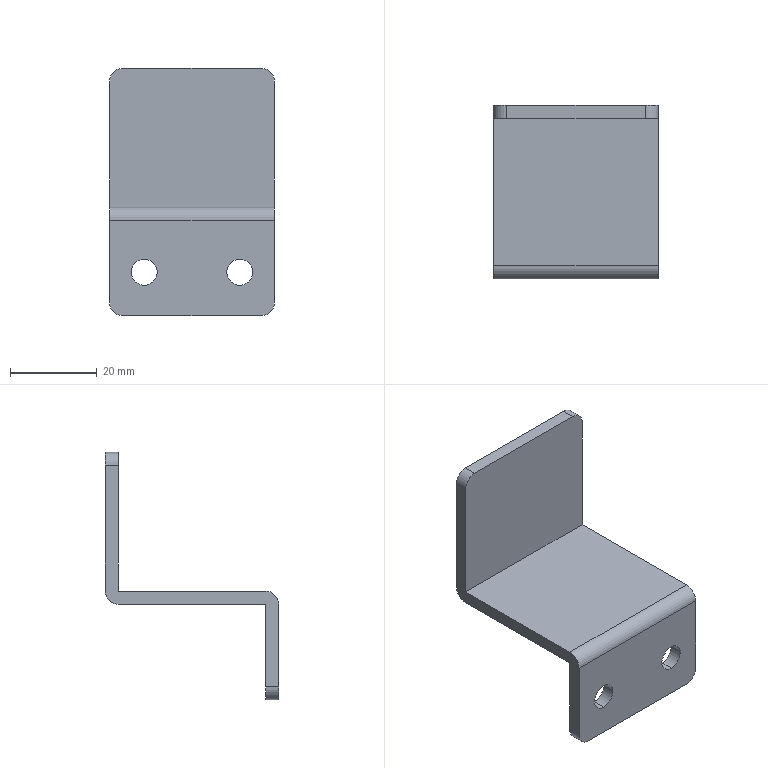Part | SolidWorks | features BaseBody 1 | 1 solid | 20 faces | box 38 x 40 x 57 mm | volume 10376 mm3 | cylinder 10 | plane 10 | commonest cylinder face diameters 6 x10
STEP:
#1=CARTESIAN_POINT('',(30.,-40.,-44.));
#2=VERTEX_POINT('',#1);
#3=CARTESIAN_POINT('',(30.,-40.,-50.));
#4=VERTEX_POINT('',#3);
#5=CARTESIAN_POINT('',(30.,-40.,-47.));
#6=DIRECTION('',(0.,-1.,0.));
#7=DIRECTION('',(0.,0.,1.));
#8=AXIS2_PLACEMENT_3D('',#5,#6,#7);
#9=CIRCLE('',#8,3.);
#10=EDGE_CURVE('',#2,#4,#9,.T.);
#11=ORIENTED_EDGE('',*,*,#10,.T.);
#12=CARTESIAN_POINT('',(30.,-37.,-50.));
#13=VERTEX_POINT('',#12);
#14=CARTESIAN_POINT('',(30.,-40.,-50.));
#15=DIRECTION('',(0.,1.,0.));
#16=VECTOR('',#15,1000.);
#17=LINE('',#14,#16);
#18=EDGE_CURVE('',#4,#13,#17,.T.);
#19=ORIENTED_EDGE('',*,*,#18,.T.);
#20=CARTESIAN_POINT('',(30.,-37.,-44.));
#21=VERTEX_POINT('',#20);
#22=CARTESIAN_POINT('',(30.,-37.,-47.));
#23=DIRECTION('',(0.,1.,0.));
#24=DIRECTION('',(0.,0.,1.));
#25=AXIS2_PLACEMENT_3D('',#22,#23,#24);
#26=CIRCLE('',#25,3.);
#27=EDGE_CURVE('',#13,#21,#26,.T.);
#28=ORIENTED_EDGE('',*,*,#27,.T.);
#29=CARTESIAN_POINT('',(30.,-40.,-44.));
#30=DIRECTION('',(0.,1.,0.));
#31=VECTOR('',#30,1000.);
#32=LINE('',#29,#31);
#33=EDGE_CURVE('',#2,#21,#32,.T.);
#34=ORIENTED_EDGE('',*,*,#33,.F.);
#35=EDGE_LOOP('',(#11,#19,#28,#34));
#36=FACE_OUTER_BOUND('',#35,.T.);
#37=CARTESIAN_POINT('',(30.,-40.,-47.));
#38=DIRECTION('',(0.,1.,0.));
#39=DIRECTION('',(0.,0.,1.));
#40=AXIS2_PLACEMENT_3D('',#37,#38,#39);
#41=CYLINDRICAL_SURFACE('',#40,3.);
#42=ADVANCED_FACE('',(#36),#41,.F.);
#43=CARTESIAN_POINT('',(8.,-40.,-44.));
#44=VERTEX_POINT('',#43);
#45=CARTESIAN_POINT('',(8.,-40.,-50.));
#46=VERTEX_POINT('',#45);
#47=CARTESIAN_POINT('',(8.,-40.,-47.));
#48=DIRECTION('',(0.,-1.,0.));
#49=DIRECTION('',(0.,0.,1.));
#50=AXIS2_PLACEMENT_3D('',#47,#48,#49);
#51=CIRCLE('',#50,3.);
#52=EDGE_CURVE('',#44,#46,#51,.T.);
#53=ORIENTED_EDGE('',*,*,#52,.T.);
#54=CARTESIAN_POINT('',(8.,-37.,-50.));
#55=VERTEX_POINT('',#54);
#56=CARTESIAN_POINT('',(8.,-40.,-50.));
#57=DIRECTION('',(0.,1.,0.));
#58=VECTOR('',#57,1000.);
#59=LINE('',#56,#58);
#60=EDGE_CURVE('',#46,#55,#59,.T.);
#61=ORIENTED_EDGE('',*,*,#60,.T.);
#62=CARTESIAN_POINT('',(8.,-37.,-44.));
#63=VERTEX_POINT('',#62);
#64=CARTESIAN_POINT('',(8.,-37.,-47.));
#65=DIRECTION('',(0.,1.,0.));
#66=DIRECTION('',(0.,0.,1.));
#67=AXIS2_PLACEMENT_3D('',#64,#65,#66);
#68=CIRCLE('',#67,3.);
#69=EDGE_CURVE('',#55,#63,#68,.T.);
#70=ORIENTED_EDGE('',*,*,#69,.T.);
#71=CARTESIAN_POINT('',(8.,-40.,-44.));
#72=DIRECTION('',(0.,1.,0.));
#73=VECTOR('',#72,1000.);
#74=LINE('',#71,#73);
#75=EDGE_CURVE('',#44,#63,#74,.T.);
#76=ORIENTED_EDGE('',*,*,#75,.F.);
#77=EDGE_LOOP('',(#53,#61,#70,#76));
#78=FACE_OUTER_BOUND('',#77,.T.);
#79=CARTESIAN_POINT('',(8.,-40.,-47.));
#80=DIRECTION('',(0.,1.,0.));
#81=DIRECTION('',(0.,0.,1.));
#82=AXIS2_PLACEMENT_3D('',#79,#80,#81);
#83=CYLINDRICAL_SURFACE('',#82,3.);
#84=ADVANCED_FACE('',(#78),#83,.F.);
#85=CARTESIAN_POINT('',(38.,-37.,-32.));
#86=VERTEX_POINT('',#85);
#87=CARTESIAN_POINT('',(0.,-37.,-32.));
#88=VERTEX_POINT('',#87);
#89=CARTESIAN_POINT('',(38.,-37.,-32.));
#90=DIRECTION('',(-1.,0.,0.));
#91=VECTOR('',#90,1000.);
#92=LINE('',#89,#91);
#93=EDGE_CURVE('',#86,#88,#92,.T.);
#94=ORIENTED_EDGE('',*,*,#93,.F.);
#95=CARTESIAN_POINT('',(38.,-3.,-32.));
#96=VERTEX_POINT('',#95);
#97=CARTESIAN_POINT('',(38.,-40.,-32.));
#98=DIRECTION('',(0.,-1.,0.));
#99=VECTOR('',#98,1000.);
#100=LINE('',#97,#99);
#101=EDGE_CURVE('',#96,#86,#100,.T.);
#102=ORIENTED_EDGE('',*,*,#101,.F.);
#103=CARTESIAN_POINT('',(0.,-3.,-32.));
#104=VERTEX_POINT('',#103);
#105=CARTESIAN_POINT('',(38.,-3.,-32.));
#106=DIRECTION('',(1.,0.,0.));
#107=VECTOR('',#106,1000.);
#108=LINE('',#105,#107);
#109=EDGE_CURVE('',#104,#96,#108,.T.);
#110=ORIENTED_EDGE('',*,*,#109,.F.);
#111=CARTESIAN_POINT('',(0.,-40.,-32.));
#112=DIRECTION('',(0.,1.,0.));
#113=VECTOR('',#112,1000.);
#114=LINE('',#111,#113);
#115=EDGE_CURVE('',#88,#104,#114,.T.);
#116=ORIENTED_EDGE('',*,*,#115,.F.);
#117=EDGE_LOOP('',(#94,#102,#110,#116));
#118=FACE_OUTER_BOUND('',#117,.T.);
#119=CARTESIAN_POINT('',(38.,-40.,-32.));
#120=DIRECTION('',(0.,0.,-1.));
#121=DIRECTION('',(0.,1.,0.));
#122=AXIS2_PLACEMENT_3D('',#119,#120,#121);
#123=PLANE('',#122);
#124=ADVANCED_FACE('',(#118),#123,.F.);
#125=CARTESIAN_POINT('',(0.,0.,-32.));
#126=VERTEX_POINT('',#125);
#127=CARTESIAN_POINT('',(0.,-3.,-35.));
#128=VERTEX_POINT('',#127);
#129=CARTESIAN_POINT('',(0.,-3.,-32.));
#130=DIRECTION('',(-1.,0.,0.));
#131=DIRECTION('',(0.,0.,1.));
#132=AXIS2_PLACEMENT_3D('',#129,#130,#131);
#133=CIRCLE('',#132,3.);
#134=EDGE_CURVE('',#126,#128,#133,.T.);
#135=ORIENTED_EDGE('',*,*,#134,.T.);
#136=CARTESIAN_POINT('',(0.,-37.,-35.));
#137=VERTEX_POINT('',#136);
#138=CARTESIAN_POINT('',(0.,0.,-35.));
#139=DIRECTION('',(0.,-1.,0.));
#140=VECTOR('',#139,1000.);
#141=LINE('',#138,#140);
#142=EDGE_CURVE('',#128,#137,#141,.T.);
#143=ORIENTED_EDGE('',*,*,#142,.T.);
#144=CARTESIAN_POINT('',(0.,-37.,-54.));
#145=VERTEX_POINT('',#144);
#146=CARTESIAN_POINT('',(0.,-37.,0.));
#147=DIRECTION('',(0.,0.,-1.));
#148=VECTOR('',#147,1000.);
#149=LINE('',#146,#148);
#150=EDGE_CURVE('',#137,#145,#149,.T.);
#151=ORIENTED_EDGE('',*,*,#150,.T.);
#152=CARTESIAN_POINT('',(0.,-40.,-54.));
#153=VERTEX_POINT('',#152);
#154=CARTESIAN_POINT('',(0.,0.,-54.));
#155=DIRECTION('',(0.,-1.,0.));
#156=VECTOR('',#155,1000.);
#157=LINE('',#154,#156);
#158=EDGE_CURVE('',#145,#153,#157,.T.);
#159=ORIENTED_EDGE('',*,*,#158,.T.);
#160=CARTESIAN_POINT('',(0.,-40.,-35.));
#161=VERTEX_POINT('',#160);
#162=CARTESIAN_POINT('',(0.,-40.,0.));
#163=DIRECTION('',(0.,0.,1.));
#164=VECTOR('',#163,1000.);
#165=LINE('',#162,#164);
#166=EDGE_CURVE('',#153,#161,#165,.T.);
#167=ORIENTED_EDGE('',*,*,#166,.T.);
#168=CARTESIAN_POINT('',(0.,-37.,-35.));
#169=DIRECTION('',(-1.,0.,0.));
#170=DIRECTION('',(0.,0.,1.));
#171=AXIS2_PLACEMENT_3D('',#168,#169,#170);
#172=CIRCLE('',#171,3.);
#173=EDGE_CURVE('',#161,#88,#172,.T.);
#174=ORIENTED_EDGE('',*,*,#173,.T.);
#175=ORIENTED_EDGE('',*,*,#115,.T.);
#176=CARTESIAN_POINT('',(0.,-3.,-3.));
#177=VERTEX_POINT('',#176);
#178=CARTESIAN_POINT('',(0.,-3.,0.));
#179=DIRECTION('',(0.,0.,1.));
#180=VECTOR('',#179,1000.);
#181=LINE('',#178,#180);
#182=EDGE_CURVE('',#104,#177,#181,.T.);
#183=ORIENTED_EDGE('',*,*,#182,.T.);
#184=CARTESIAN_POINT('',(0.,0.,-3.));
#185=VERTEX_POINT('',#184);
#186=CARTESIAN_POINT('',(0.,0.,-3.));
#187=DIRECTION('',(0.,1.,0.));
#188=VECTOR('',#187,1000.);
#189=LINE('',#186,#188);
#190=EDGE_CURVE('',#177,#185,#189,.T.);
#191=ORIENTED_EDGE('',*,*,#190,.T.);
#192=CARTESIAN_POINT('',(0.,0.,0.));
#193=DIRECTION('',(0.,0.,-1.));
#194=VECTOR('',#193,1000.);
#195=LINE('',#192,#194);
#196=EDGE_CURVE('',#185,#126,#195,.T.);
#197=ORIENTED_EDGE('',*,*,#196,.T.);
#198=EDGE_LOOP('',(#135,#143,#151,#159,#167,#174,#175,#183,#191,#197));
#199=FACE_OUTER_BOUND('',#198,.T.);
#200=CARTESIAN_POINT('',(0.,0.,0.));
#201=DIRECTION('',(-1.,0.,0.));
#202=DIRECTION('',(0.,0.,1.));
#203=AXIS2_PLACEMENT_3D('',#200,#201,#202);
#204=PLANE('',#203);
#205=ADVANCED_FACE('',(#199),#204,.T.);
#206=ORIENTED_EDGE('',*,*,#173,.F.);
#207=CARTESIAN_POINT('',(38.,-40.,-35.));
#208=VERTEX_POINT('',#207);
#209=CARTESIAN_POINT('',(38.,-40.,-35.));
#210=DIRECTION('',(1.,0.,0.));
#211=VECTOR('',#210,1000.);
#212=LINE('',#209,#211);
#213=EDGE_CURVE('',#161,#208,#212,.T.);
#214=ORIENTED_EDGE('',*,*,#213,.T.);
#215=CARTESIAN_POINT('',(38.,-37.,-35.));
#216=DIRECTION('',(-1.,0.,0.));
#217=DIRECTION('',(0.,0.,1.));
#218=AXIS2_PLACEMENT_3D('',#215,#216,#217);
#219=CIRCLE('',#218,3.);
#220=EDGE_CURVE('',#208,#86,#219,.T.);
#221=ORIENTED_EDGE('',*,*,#220,.T.);
#222=ORIENTED_EDGE('',*,*,#93,.T.);
#223=EDGE_LOOP('',(#206,#214,#221,#222));
#224=FACE_OUTER_BOUND('',#223,.T.);
#225=CARTESIAN_POINT('',(38.,-37.,-35.));
#226=DIRECTION('',(-1.,0.,0.));
#227=DIRECTION('',(0.,0.,1.));
#228=AXIS2_PLACEMENT_3D('',#225,#226,#227);
#229=CYLINDRICAL_SURFACE('',#228,3.);
#230=ADVANCED_FACE('',(#224),#229,.T.);
#231=CARTESIAN_POINT('',(38.,-37.,-54.));
#232=VERTEX_POINT('',#231);
#233=CARTESIAN_POINT('',(38.,-40.,-54.));
#234=VERTEX_POINT('',#233);
#235=CARTESIAN_POINT('',(38.,0.,-54.));
#236=DIRECTION('',(0.,-1.,0.));
#237=VECTOR('',#236,1000.);
#238=LINE('',#235,#237);
#239=EDGE_CURVE('',#232,#234,#238,.T.);
#240=ORIENTED_EDGE('',*,*,#239,.F.);
#241=CARTESIAN_POINT('',(38.,-37.,-35.));
#242=VERTEX_POINT('',#241);
#243=CARTESIAN_POINT('',(38.,-37.,0.));
#244=DIRECTION('',(0.,0.,-1.));
#245=VECTOR('',#244,1000.);
#246=LINE('',#243,#245);
#247=EDGE_CURVE('',#242,#232,#246,.T.);
#248=ORIENTED_EDGE('',*,*,#247,.F.);
#249=CARTESIAN_POINT('',(38.,-3.,-35.));
#250=VERTEX_POINT('',#249);
#251=CARTESIAN_POINT('',(38.,0.,-35.));
#252=DIRECTION('',(0.,-1.,0.));
#253=VECTOR('',#252,1000.);
#254=LINE('',#251,#253);
#255=EDGE_CURVE('',#250,#242,#254,.T.);
#256=ORIENTED_EDGE('',*,*,#255,.F.);
#257=CARTESIAN_POINT('',(38.,0.,-32.));
#258=VERTEX_POINT('',#257);
#259=CARTESIAN_POINT('',(38.,-3.,-32.));
#260=DIRECTION('',(-1.,0.,0.));
#261=DIRECTION('',(0.,0.,1.));
#262=AXIS2_PLACEMENT_3D('',#259,#260,#261);
#263=CIRCLE('',#262,3.);
#264=EDGE_CURVE('',#258,#250,#263,.T.);
#265=ORIENTED_EDGE('',*,*,#264,.F.);
#266=CARTESIAN_POINT('',(38.,0.,-3.));
#267=VERTEX_POINT('',#266);
#268=CARTESIAN_POINT('',(38.,0.,0.));
#269=DIRECTION('',(0.,0.,-1.));
#270=VECTOR('',#269,1000.);
#271=LINE('',#268,#270);
#272=EDGE_CURVE('',#267,#258,#271,.T.);
#273=ORIENTED_EDGE('',*,*,#272,.F.);
#274=CARTESIAN_POINT('',(38.,-3.,-3.));
#275=VERTEX_POINT('',#274);
#276=CARTESIAN_POINT('',(38.,0.,-3.));
#277=DIRECTION('',(0.,1.,0.));
#278=VECTOR('',#277,1000.);
#279=LINE('',#276,#278);
#280=EDGE_CURVE('',#275,#267,#279,.T.);
#281=ORIENTED_EDGE('',*,*,#280,.F.);
#282=CARTESIAN_POINT('',(38.,-3.,0.));
#283=DIRECTION('',(0.,0.,1.));
#284=VECTOR('',#283,1000.);
#285=LINE('',#282,#284);
#286=EDGE_CURVE('',#96,#275,#285,.T.);
#287=ORIENTED_EDGE('',*,*,#286,.F.);
#288=ORIENTED_EDGE('',*,*,#101,.T.);
#289=ORIENTED_EDGE('',*,*,#220,.F.);
#290=CARTESIAN_POINT('',(38.,-40.,0.));
#291=DIRECTION('',(0.,0.,1.));
#292=VECTOR('',#291,1000.);
#293=LINE('',#290,#292);
#294=EDGE_CURVE('',#234,#208,#293,.T.);
#295=ORIENTED_EDGE('',*,*,#294,.F.);
#296=EDGE_LOOP('',(#240,#248,#256,#265,#273,#281,#287,#288,#289,#295));
#297=FACE_OUTER_BOUND('',#296,.T.);
#298=CARTESIAN_POINT('',(38.,0.,0.));
#299=DIRECTION('',(-1.,0.,0.));
#300=DIRECTION('',(0.,0.,1.));
#301=AXIS2_PLACEMENT_3D('',#298,#299,#300);
#302=PLANE('',#301);
#303=ADVANCED_FACE('',(#297),#302,.F.);
#304=CARTESIAN_POINT('',(35.,-3.,0.));
#305=VERTEX_POINT('',#304);
#306=CARTESIAN_POINT('',(35.,-3.,-3.));
#307=DIRECTION('',(0.,1.,0.));
#308=DIRECTION('',(0.,0.,-1.));
#309=AXIS2_PLACEMENT_3D('',#306,#307,#308);
#310=CIRCLE('',#309,3.);
#311=EDGE_CURVE('',#305,#275,#310,.T.);
#312=ORIENTED_EDGE('',*,*,#311,.F.);
#313=CARTESIAN_POINT('',(3.,-3.,0.));
#314=VERTEX_POINT('',#313);
#315=CARTESIAN_POINT('',(38.,-3.,0.));
#316=DIRECTION('',(1.,0.,0.));
#317=VECTOR('',#316,1000.);
#318=LINE('',#315,#317);
#319=EDGE_CURVE('',#314,#305,#318,.T.);
#320=ORIENTED_EDGE('',*,*,#319,.F.);
#321=CARTESIAN_POINT('',(3.,-3.,-3.));
#322=DIRECTION('',(0.,1.,0.));
#323=DIRECTION('',(0.,0.,1.));
#324=AXIS2_PLACEMENT_3D('',#321,#322,#323);
#325=CIRCLE('',#324,3.);
#326=EDGE_CURVE('',#177,#314,#325,.T.);
#327=ORIENTED_EDGE('',*,*,#326,.F.);
#328=ORIENTED_EDGE('',*,*,#182,.F.);
#329=ORIENTED_EDGE('',*,*,#109,.T.);
#330=ORIENTED_EDGE('',*,*,#286,.T.);
#331=EDGE_LOOP('',(#312,#320,#327,#328,#329,#330));
#332=FACE_OUTER_BOUND('',#331,.T.);
#333=CARTESIAN_POINT('',(38.,-3.,-32.));
#334=DIRECTION('',(0.,1.,0.));
#335=DIRECTION('',(0.,0.,1.));
#336=AXIS2_PLACEMENT_3D('',#333,#334,#335);
#337=PLANE('',#336);
#338=ADVANCED_FACE('',(#332),#337,.F.);
#339=CARTESIAN_POINT('',(38.,-3.,-35.));
#340=DIRECTION('',(-1.,0.,0.));
#341=VECTOR('',#340,1000.);
#342=LINE('',#339,#341);
#343=EDGE_CURVE('',#250,#128,#342,.T.);
#344=ORIENTED_EDGE('',*,*,#343,.F.);
#345=ORIENTED_EDGE('',*,*,#255,.T.);
#346=CARTESIAN_POINT('',(38.,-37.,-35.));
#347=DIRECTION('',(1.,0.,0.));
#348=VECTOR('',#347,1000.);
#349=LINE('',#346,#348);
#350=EDGE_CURVE('',#137,#242,#349,.T.);
#351=ORIENTED_EDGE('',*,*,#350,.F.);
#352=ORIENTED_EDGE('',*,*,#142,.F.);
#353=EDGE_LOOP('',(#344,#345,#351,#352));
#354=FACE_OUTER_BOUND('',#353,.T.);
#355=CARTESIAN_POINT('',(38.,0.,-35.));
#356=DIRECTION('',(0.,0.,1.));
#357=DIRECTION('',(0.,-1.,0.));
#358=AXIS2_PLACEMENT_3D('',#355,#356,#357);
#359=PLANE('',#358);
#360=ADVANCED_FACE('',(#354),#359,.F.);
#361=ORIENTED_EDGE('',*,*,#134,.F.);
#362=CARTESIAN_POINT('',(38.,0.,-32.));
#363=DIRECTION('',(1.,0.,0.));
#364=VECTOR('',#363,1000.);
#365=LINE('',#362,#364);
#366=EDGE_CURVE('',#126,#258,#365,.T.);
#367=ORIENTED_EDGE('',*,*,#366,.T.);
#368=ORIENTED_EDGE('',*,*,#264,.T.);
#369=ORIENTED_EDGE('',*,*,#343,.T.);
#370=EDGE_LOOP('',(#361,#367,#368,#369));
#371=FACE_OUTER_BOUND('',#370,.T.);
#372=CARTESIAN_POINT('',(38.,-3.,-32.));
#373=DIRECTION('',(-1.,0.,0.));
#374=DIRECTION('',(0.,0.,1.));
#375=AXIS2_PLACEMENT_3D('',#372,#373,#374);
#376=CYLINDRICAL_SURFACE('',#375,3.);
#377=ADVANCED_FACE('',(#371),#376,.T.);
#378=CARTESIAN_POINT('',(35.,0.,0.));
#379=VERTEX_POINT('',#378);
#380=CARTESIAN_POINT('',(35.,0.,-3.));
#381=DIRECTION('',(0.,-1.,0.));
#382=DIRECTION('',(0.,0.,-1.));
#383=AXIS2_PLACEMENT_3D('',#380,#381,#382);
#384=CIRCLE('',#383,3.);
#385=EDGE_CURVE('',#267,#379,#384,.T.);
#386=ORIENTED_EDGE('',*,*,#385,.F.);
#387=ORIENTED_EDGE('',*,*,#272,.T.);
#388=ORIENTED_EDGE('',*,*,#366,.F.);
#389=ORIENTED_EDGE('',*,*,#196,.F.);
#390=CARTESIAN_POINT('',(3.,0.,0.));
#391=VERTEX_POINT('',#390);
#392=CARTESIAN_POINT('',(3.,0.,-3.));
#393=DIRECTION('',(0.,-1.,0.));
#394=DIRECTION('',(0.,0.,1.));
#395=AXIS2_PLACEMENT_3D('',#392,#393,#394);
#396=CIRCLE('',#395,3.);
#397=EDGE_CURVE('',#391,#185,#396,.T.);
#398=ORIENTED_EDGE('',*,*,#397,.F.);
#399=CARTESIAN_POINT('',(38.,0.,0.));
#400=DIRECTION('',(-1.,0.,0.));
#401=VECTOR('',#400,1000.);
#402=LINE('',#399,#401);
#403=EDGE_CURVE('',#379,#391,#402,.T.);
#404=ORIENTED_EDGE('',*,*,#403,.F.);
#405=EDGE_LOOP('',(#386,#387,#388,#389,#398,#404));
#406=FACE_OUTER_BOUND('',#405,.T.);
#407=CARTESIAN_POINT('',(38.,0.,0.));
#408=DIRECTION('',(0.,-1.,0.));
#409=DIRECTION('',(0.,0.,-1.));
#410=AXIS2_PLACEMENT_3D('',#407,#408,#409);
#411=PLANE('',#410);
#412=ADVANCED_FACE('',(#406),#411,.F.);
#413=ORIENTED_EDGE('',*,*,#326,.T.);
#414=CARTESIAN_POINT('',(3.,-3.,0.));
#415=DIRECTION('',(0.,1.,0.));
#416=VECTOR('',#415,1000.);
#417=LINE('',#414,#416);
#418=EDGE_CURVE('',#314,#391,#417,.T.);
#419=ORIENTED_EDGE('',*,*,#418,.T.);
#420=ORIENTED_EDGE('',*,*,#397,.T.);
#421=ORIENTED_EDGE('',*,*,#190,.F.);
#422=EDGE_LOOP('',(#413,#419,#420,#421));
#423=FACE_OUTER_BOUND('',#422,.T.);
#424=CARTESIAN_POINT('',(3.,-3.,-3.));
#425=DIRECTION('',(0.,1.,0.));
#426=DIRECTION('',(0.,0.,1.));
#427=AXIS2_PLACEMENT_3D('',#424,#425,#426);
#428=CYLINDRICAL_SURFACE('',#427,3.);
#429=ADVANCED_FACE('',(#423),#428,.T.);
#430=CARTESIAN_POINT('',(3.,-40.,-57.));
#431=VERTEX_POINT('',#430);
#432=CARTESIAN_POINT('',(3.,-40.,-54.));
#433=DIRECTION('',(0.,1.,0.));
#434=DIRECTION('',(0.,0.,-1.));
#435=AXIS2_PLACEMENT_3D('',#432,#433,#434);
#436=CIRCLE('',#435,3.);
#437=EDGE_CURVE('',#431,#153,#436,.T.);
#438=ORIENTED_EDGE('',*,*,#437,.F.);
#439=CARTESIAN_POINT('',(35.,-40.,-57.));
#440=VERTEX_POINT('',#439);
#441=CARTESIAN_POINT('',(38.,-40.,-57.));
#442=DIRECTION('',(-1.,0.,0.));
#443=VECTOR('',#442,1000.);
#444=LINE('',#441,#443);
#445=EDGE_CURVE('',#440,#431,#444,.T.);
#446=ORIENTED_EDGE('',*,*,#445,.F.);
#447=CARTESIAN_POINT('',(35.,-40.,-54.));
#448=DIRECTION('',(0.,1.,0.));
#449=DIRECTION('',(0.,0.,1.));
#450=AXIS2_PLACEMENT_3D('',#447,#448,#449);
#451=CIRCLE('',#450,3.);
#452=EDGE_CURVE('',#234,#440,#451,.T.);
#453=ORIENTED_EDGE('',*,*,#452,.F.);
#454=ORIENTED_EDGE('',*,*,#294,.T.);
#455=ORIENTED_EDGE('',*,*,#213,.F.);
#456=ORIENTED_EDGE('',*,*,#166,.F.);
#457=EDGE_LOOP('',(#438,#446,#453,#454,#455,#456));
#458=FACE_OUTER_BOUND('',#457,.T.);
#459=ORIENTED_EDGE('',*,*,#10,.F.);
#460=CARTESIAN_POINT('',(30.,-40.,-47.));
#461=DIRECTION('',(0.,-1.,0.));
#462=DIRECTION('',(0.,0.,1.));
#463=AXIS2_PLACEMENT_3D('',#460,#461,#462);
#464=CIRCLE('',#463,3.);
#465=EDGE_CURVE('',#4,#2,#464,.T.);
#466=ORIENTED_EDGE('',*,*,#465,.F.);
#467=EDGE_LOOP('',(#459,#466));
#468=FACE_BOUND('',#467,.T.);
#469=ORIENTED_EDGE('',*,*,#52,.F.);
#470=CARTESIAN_POINT('',(8.,-40.,-47.));
#471=DIRECTION('',(0.,-1.,0.));
#472=DIRECTION('',(0.,0.,1.));
#473=AXIS2_PLACEMENT_3D('',#470,#471,#472);
#474=CIRCLE('',#473,3.);
#475=EDGE_CURVE('',#46,#44,#474,.T.);
#476=ORIENTED_EDGE('',*,*,#475,.F.);
#477=EDGE_LOOP('',(#469,#476));
#478=FACE_BOUND('',#477,.T.);
#479=CARTESIAN_POINT('',(38.,-40.,-57.));
#480=DIRECTION('',(0.,1.,0.));
#481=DIRECTION('',(0.,0.,1.));
#482=AXIS2_PLACEMENT_3D('',#479,#480,#481);
#483=PLANE('',#482);
#484=ADVANCED_FACE('',(#458,#468,#478),#483,.F.);
#485=CARTESIAN_POINT('',(3.,-37.,-57.));
#486=VERTEX_POINT('',#485);
#487=CARTESIAN_POINT('',(3.,-37.,-54.));
#488=DIRECTION('',(0.,-1.,0.));
#489=DIRECTION('',(0.,0.,-1.));
#490=AXIS2_PLACEMENT_3D('',#487,#488,#489);
#491=CIRCLE('',#490,3.);
#492=EDGE_CURVE('',#145,#486,#491,.T.);
#493=ORIENTED_EDGE('',*,*,#492,.T.);
#494=CARTESIAN_POINT('',(3.,-37.,-57.));
#495=DIRECTION('',(0.,-1.,0.));
#496=VECTOR('',#495,1000.);
#497=LINE('',#494,#496);
#498=EDGE_CURVE('',#486,#431,#497,.T.);
#499=ORIENTED_EDGE('',*,*,#498,.T.);
#500=ORIENTED_EDGE('',*,*,#437,.T.);
#501=ORIENTED_EDGE('',*,*,#158,.F.);
#502=EDGE_LOOP('',(#493,#499,#500,#501));
#503=FACE_OUTER_BOUND('',#502,.T.);
#504=CARTESIAN_POINT('',(3.,-37.,-54.));
#505=DIRECTION('',(0.,-1.,0.));
#506=DIRECTION('',(0.,0.,-1.));
#507=AXIS2_PLACEMENT_3D('',#504,#505,#506);
#508=CYLINDRICAL_SURFACE('',#507,3.);
#509=ADVANCED_FACE('',(#503),#508,.T.);
#510=ORIENTED_EDGE('',*,*,#492,.F.);
#511=ORIENTED_EDGE('',*,*,#150,.F.);
#512=ORIENTED_EDGE('',*,*,#350,.T.);
#513=ORIENTED_EDGE('',*,*,#247,.T.);
#514=CARTESIAN_POINT('',(35.,-37.,-57.));
#515=VERTEX_POINT('',#514);
#516=CARTESIAN_POINT('',(35.,-37.,-54.));
#517=DIRECTION('',(0.,-1.,0.));
#518=DIRECTION('',(0.,0.,1.));
#519=AXIS2_PLACEMENT_3D('',#516,#517,#518);
#520=CIRCLE('',#519,3.);
#521=EDGE_CURVE('',#515,#232,#520,.T.);
#522=ORIENTED_EDGE('',*,*,#521,.F.);
#523=CARTESIAN_POINT('',(38.,-37.,-57.));
#524=DIRECTION('',(1.,0.,0.));
#525=VECTOR('',#524,1000.);
#526=LINE('',#523,#525);
#527=EDGE_CURVE('',#486,#515,#526,.T.);
#528=ORIENTED_EDGE('',*,*,#527,.F.);
#529=EDGE_LOOP('',(#510,#511,#512,#513,#522,#528));
#530=FACE_OUTER_BOUND('',#529,.T.);
#531=CARTESIAN_POINT('',(30.,-37.,-47.));
#532=DIRECTION('',(0.,1.,0.));
#533=DIRECTION('',(0.,0.,1.));
#534=AXIS2_PLACEMENT_3D('',#531,#532,#533);
#535=CIRCLE('',#534,3.);
#536=EDGE_CURVE('',#21,#13,#535,.T.);
#537=ORIENTED_EDGE('',*,*,#536,.F.);
#538=ORIENTED_EDGE('',*,*,#27,.F.);
#539=EDGE_LOOP('',(#537,#538));
#540=FACE_BOUND('',#539,.T.);
#541=CARTESIAN_POINT('',(8.,-37.,-47.));
#542=DIRECTION('',(0.,1.,0.));
#543=DIRECTION('',(0.,0.,1.));
#544=AXIS2_PLACEMENT_3D('',#541,#542,#543);
#545=CIRCLE('',#544,3.);
#546=EDGE_CURVE('',#63,#55,#545,.T.);
#547=ORIENTED_EDGE('',*,*,#546,.F.);
#548=ORIENTED_EDGE('',*,*,#69,.F.);
#549=EDGE_LOOP('',(#547,#548));
#550=FACE_BOUND('',#549,.T.);
#551=CARTESIAN_POINT('',(38.,-37.,-35.));
#552=DIRECTION('',(0.,-1.,0.));
#553=DIRECTION('',(0.,0.,-1.));
#554=AXIS2_PLACEMENT_3D('',#551,#552,#553);
#555=PLANE('',#554);
#556=ADVANCED_FACE('',(#530,#540,#550),#555,.F.);
#557=ORIENTED_EDGE('',*,*,#521,.T.);
#558=ORIENTED_EDGE('',*,*,#239,.T.);
#559=ORIENTED_EDGE('',*,*,#452,.T.);
#560=CARTESIAN_POINT('',(35.,0.,-57.));
#561=DIRECTION('',(0.,1.,0.));
#562=VECTOR('',#561,1000.);
#563=LINE('',#560,#562);
#564=EDGE_CURVE('',#440,#515,#563,.T.);
#565=ORIENTED_EDGE('',*,*,#564,.T.);
#566=EDGE_LOOP('',(#557,#558,#559,#565));
#567=FACE_OUTER_BOUND('',#566,.T.);
#568=CARTESIAN_POINT('',(35.,0.,-54.));
#569=DIRECTION('',(0.,1.,0.));
#570=DIRECTION('',(0.,0.,1.));
#571=AXIS2_PLACEMENT_3D('',#568,#569,#570);
#572=CYLINDRICAL_SURFACE('',#571,3.);
#573=ADVANCED_FACE('',(#567),#572,.T.);
#574=ORIENTED_EDGE('',*,*,#311,.T.);
#575=ORIENTED_EDGE('',*,*,#280,.T.);
#576=ORIENTED_EDGE('',*,*,#385,.T.);
#577=CARTESIAN_POINT('',(35.,0.,0.));
#578=DIRECTION('',(0.,-1.,0.));
#579=VECTOR('',#578,1000.);
#580=LINE('',#577,#579);
#581=EDGE_CURVE('',#379,#305,#580,.T.);
#582=ORIENTED_EDGE('',*,*,#581,.T.);
#583=EDGE_LOOP('',(#574,#575,#576,#582));
#584=FACE_OUTER_BOUND('',#583,.T.);
#585=CARTESIAN_POINT('',(35.,0.,-3.));
#586=DIRECTION('',(0.,-1.,0.));
#587=DIRECTION('',(0.,0.,-1.));
#588=AXIS2_PLACEMENT_3D('',#585,#586,#587);
#589=CYLINDRICAL_SURFACE('',#588,3.);
#590=ADVANCED_FACE('',(#584),#589,.T.);
#591=ORIENTED_EDGE('',*,*,#581,.F.);
#592=ORIENTED_EDGE('',*,*,#403,.T.);
#593=ORIENTED_EDGE('',*,*,#418,.F.);
#594=ORIENTED_EDGE('',*,*,#319,.T.);
#595=EDGE_LOOP('',(#591,#592,#593,#594));
#596=FACE_OUTER_BOUND('',#595,.T.);
#597=CARTESIAN_POINT('',(38.,-3.,0.));
#598=DIRECTION('',(0.,0.,-1.));
#599=DIRECTION('',(-1.,0.,0.));
#600=AXIS2_PLACEMENT_3D('',#597,#598,#599);
#601=PLANE('',#600);
#602=ADVANCED_FACE('',(#596),#601,.F.);
#603=ORIENTED_EDGE('',*,*,#498,.F.);
#604=ORIENTED_EDGE('',*,*,#527,.T.);
#605=ORIENTED_EDGE('',*,*,#564,.F.);
#606=ORIENTED_EDGE('',*,*,#445,.T.);
#607=EDGE_LOOP('',(#603,#604,#605,#606));
#608=FACE_OUTER_BOUND('',#607,.T.);
#609=CARTESIAN_POINT('',(38.,-37.,-57.));
#610=DIRECTION('',(0.,0.,1.));
#611=DIRECTION('',(1.,0.,0.));
#612=AXIS2_PLACEMENT_3D('',#609,#610,#611);
#613=PLANE('',#612);
#614=ADVANCED_FACE('',(#608),#613,.F.);
#615=ORIENTED_EDGE('',*,*,#18,.F.);
#616=ORIENTED_EDGE('',*,*,#465,.T.);
#617=ORIENTED_EDGE('',*,*,#33,.T.);
#618=ORIENTED_EDGE('',*,*,#536,.T.);
#619=EDGE_LOOP('',(#615,#616,#617,#618));
#620=FACE_OUTER_BOUND('',#619,.T.);
#621=CARTESIAN_POINT('',(30.,-40.,-47.));
#622=DIRECTION('',(0.,1.,0.));
#623=DIRECTION('',(0.,0.,1.));
#624=AXIS2_PLACEMENT_3D('',#621,#622,#623);
#625=CYLINDRICAL_SURFACE('',#624,3.);
#626=ADVANCED_FACE('',(#620),#625,.F.);
#627=ORIENTED_EDGE('',*,*,#60,.F.);
#628=ORIENTED_EDGE('',*,*,#475,.T.);
#629=ORIENTED_EDGE('',*,*,#75,.T.);
#630=ORIENTED_EDGE('',*,*,#546,.T.);
#631=EDGE_LOOP('',(#627,#628,#629,#630));
#632=FACE_OUTER_BOUND('',#631,.T.);
#633=CARTESIAN_POINT('',(8.,-40.,-47.));
#634=DIRECTION('',(0.,1.,0.));
#635=DIRECTION('',(0.,0.,1.));
#636=AXIS2_PLACEMENT_3D('',#633,#634,#635);
#637=CYLINDRICAL_SURFACE('',#636,3.);
#638=ADVANCED_FACE('',(#632),#637,.F.);
#639=CLOSED_SHELL('',(#42,#84,#124,#205,#230,#303,#338,#360,#377,#412,#429,#484,#509,#556,#573,#590,#602,#614,#626,#638));
#640=MANIFOLD_SOLID_BREP('',#639);
#641=CARTESIAN_POINT('',(0.,0.,0.));
#642=DIRECTION('',(0.,0.,1.));
#643=DIRECTION('',(1.,0.,0.));
#644=AXIS2_PLACEMENT_3D('',#641,#642,#643);
#645=(LENGTH_UNIT()NAMED_UNIT(*)SI_UNIT(.MILLI.,.METRE.));
#646=UNCERTAINTY_MEASURE_WITH_UNIT(LENGTH_MEASURE(0.00001),#645,'','');
#647=(NAMED_UNIT(*)PLANE_ANGLE_UNIT()SI_UNIT($,.RADIAN.));
#648=(NAMED_UNIT(*)SI_UNIT($,.STERADIAN.)SOLID_ANGLE_UNIT());
#649=(GEOMETRIC_REPRESENTATION_CONTEXT(3)GLOBAL_UNCERTAINTY_ASSIGNED_CONTEXT((#646))GLOBAL_UNIT_ASSIGNED_CONTEXT((#645,#647,#648))REPRESENTATION_CONTEXT('',''));
#650=ADVANCED_BREP_SHAPE_REPRESENTATION('',(#640,#644),#649);